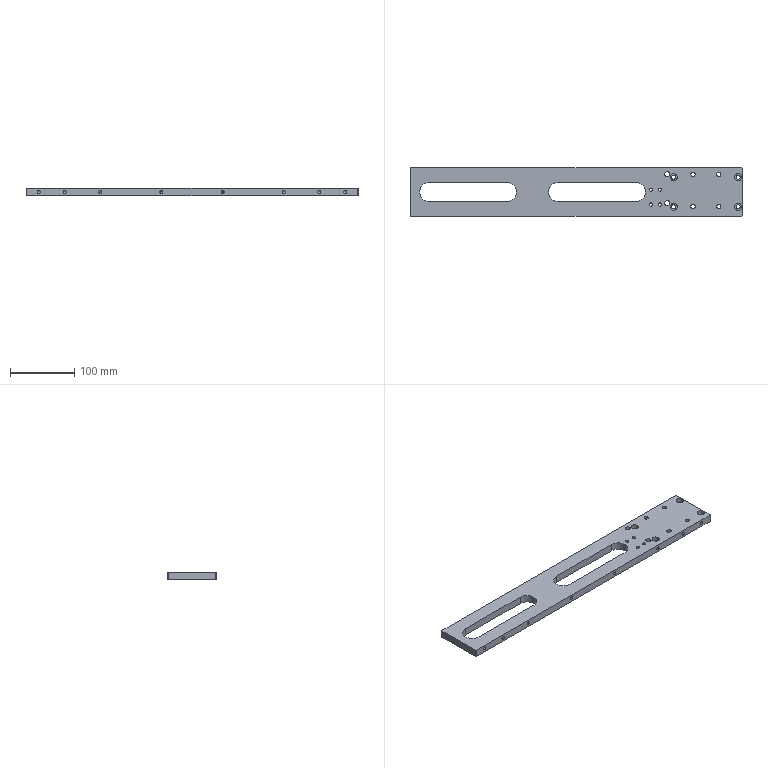Part | SolidWorks | features HoleWzd 7, Chamfer 1, Extrusion 1, ICE 1 | 1 solid | 110 faces | box 515 x 75 x 12 mm | volume 349062 mm3 | cylinder 70 | plane 24 | cone 16 | commonest cylinder face diameters 5 x28 11 x16 6.2 x8 6.6 x8 30 x6 8 x4